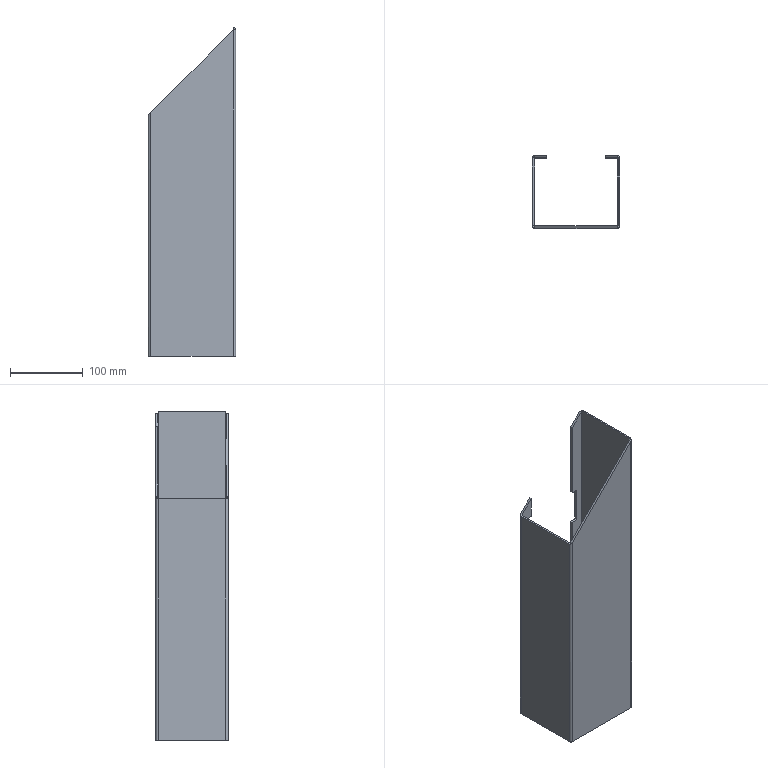Part | STEP file | TS-019-01 | 1 solid | 57 faces | box 120 x 100 x 453 mm | volume 401974 mm3 | plane 45 | cylinder 8 | spline 4 | commonest cylinder face diameters 0.4 x4 6.4 x4